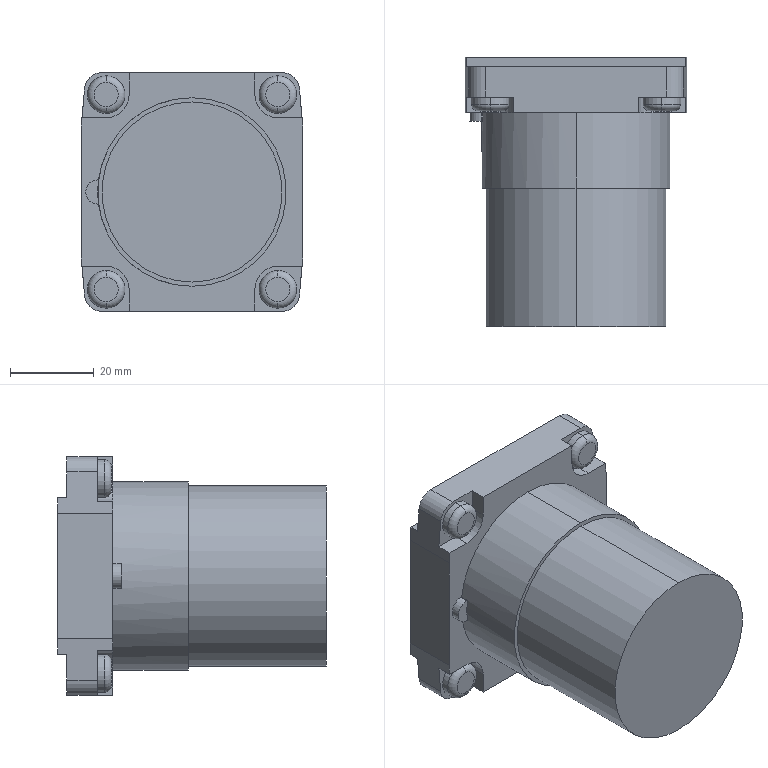Part | STEP file | _AR30-A_BONNET | 1 solid | 64 faces | box 53 x 64.2 x 57 mm | volume 112882 mm3 | plane 35 | cylinder 21 | torus 8 | commonest cylinder face diameters 9 x8 8 x4 11 x4 43 x2 45 x2 5.8 x1